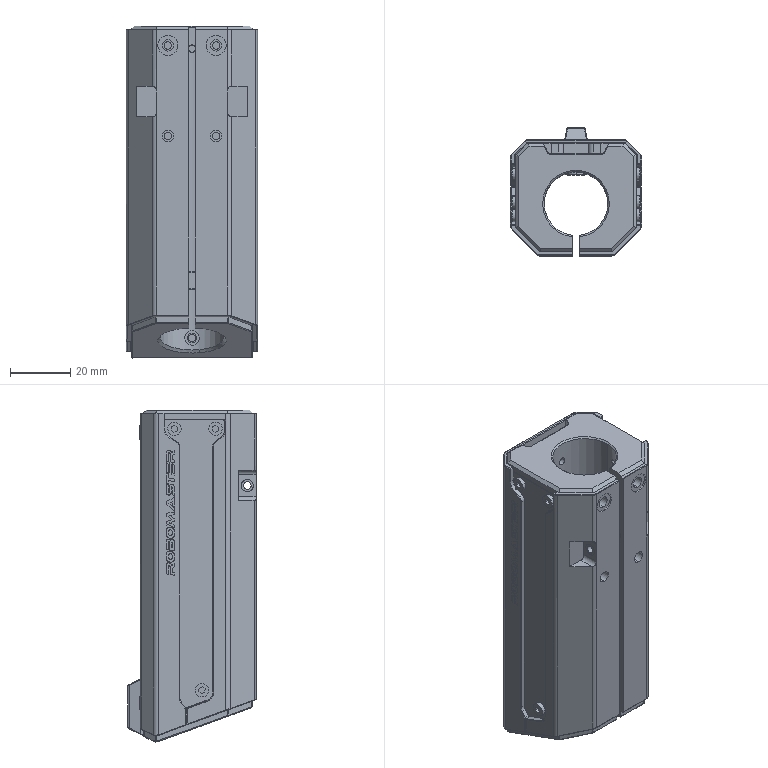Part | SolidWorks | features BaseBody 32 | 26 solids | 1341 faces | box 43.4 x 42.4 x 109.827 mm | volume 92437 mm3 | plane 702 | cylinder 447 | spline 128 | cone 64 | commonest cylinder face diameters 3.8 x66 3.2 x55 4 x53 2 x50 2.5 x30 2.37 x22